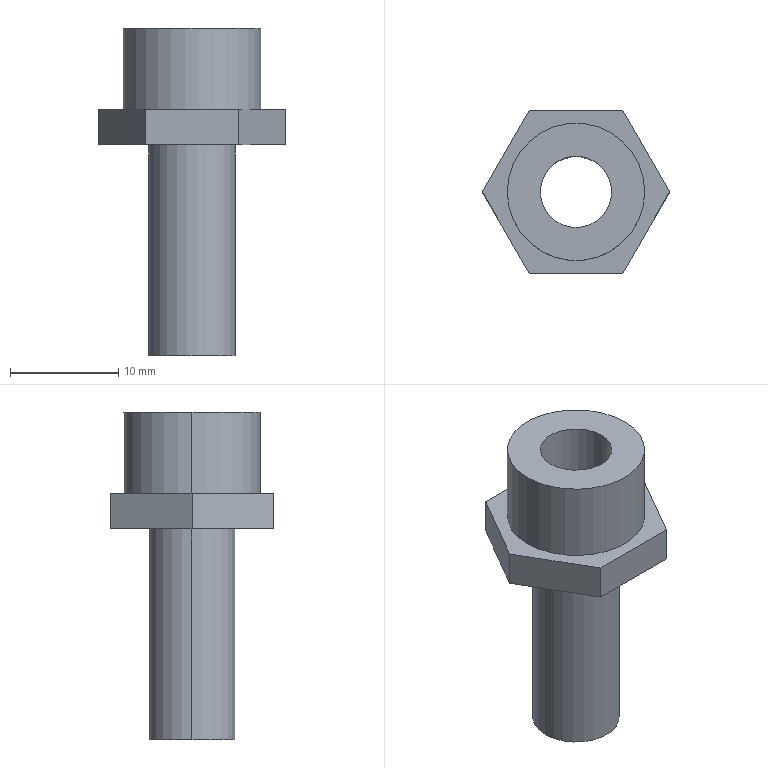Part | STEP file | 2 fen male thread×8mm | 1 solid | 16 faces | box 17.321 x 15 x 30.3 mm | volume 1537 mm3 | plane 10 | cylinder 6 | commonest cylinder face diameters 6.6 x2 8 x2 12.7 x2
STEP:
#1=CARTESIAN_POINT('',(3.3,0.,10.8));
#2=VERTEX_POINT('',#1);
#3=CARTESIAN_POINT('',(-3.3,0.,10.8));
#4=VERTEX_POINT('',#3);
#5=CARTESIAN_POINT('',(0.,0.,10.8));
#6=DIRECTION('',(0.,0.,-1.));
#7=DIRECTION('',(1.,0.,0.));
#8=AXIS2_PLACEMENT_3D('',#5,#6,#7);
#9=CIRCLE('',#8,3.3);
#10=EDGE_CURVE('',#2,#4,#9,.T.);
#11=ORIENTED_EDGE('',*,*,#10,.F.);
#12=CARTESIAN_POINT('',(3.3,0.,-19.5));
#13=VERTEX_POINT('',#12);
#14=CARTESIAN_POINT('',(3.3,0.,10.801));
#15=DIRECTION('',(0.,0.,-1.));
#16=VECTOR('',#15,1000.);
#17=LINE('',#14,#16);
#18=EDGE_CURVE('',#2,#13,#17,.T.);
#19=ORIENTED_EDGE('',*,*,#18,.T.);
#20=CARTESIAN_POINT('',(-3.3,0.,-19.5));
#21=VERTEX_POINT('',#20);
#22=CARTESIAN_POINT('',(0.,0.,-19.5));
#23=DIRECTION('',(0.,0.,-1.));
#24=DIRECTION('',(-1.,0.,0.));
#25=AXIS2_PLACEMENT_3D('',#22,#23,#24);
#26=CIRCLE('',#25,3.3);
#27=EDGE_CURVE('',#13,#21,#26,.T.);
#28=ORIENTED_EDGE('',*,*,#27,.T.);
#29=CARTESIAN_POINT('',(-3.3,0.,10.801));
#30=DIRECTION('',(0.,0.,-1.));
#31=VECTOR('',#30,1000.);
#32=LINE('',#29,#31);
#33=EDGE_CURVE('',#4,#21,#32,.T.);
#34=ORIENTED_EDGE('',*,*,#33,.F.);
#35=EDGE_LOOP('',(#11,#19,#28,#34));
#36=FACE_OUTER_BOUND('',#35,.T.);
#37=CARTESIAN_POINT('',(0.,0.,10.801));
#38=DIRECTION('',(0.,0.,-1.));
#39=DIRECTION('',(-1.,0.,0.));
#40=AXIS2_PLACEMENT_3D('',#37,#38,#39);
#41=CYLINDRICAL_SURFACE('',#40,3.3);
#42=ADVANCED_FACE('',(#36),#41,.F.);
#43=CARTESIAN_POINT('',(-4.,0.,-19.5));
#44=VERTEX_POINT('',#43);
#45=CARTESIAN_POINT('',(4.,0.,-19.5));
#46=VERTEX_POINT('',#45);
#47=CARTESIAN_POINT('',(0.,0.,-19.5));
#48=DIRECTION('',(0.,0.,-1.));
#49=DIRECTION('',(-1.,0.,0.));
#50=AXIS2_PLACEMENT_3D('',#47,#48,#49);
#51=CIRCLE('',#50,4.);
#52=EDGE_CURVE('',#44,#46,#51,.T.);
#53=ORIENTED_EDGE('',*,*,#52,.F.);
#54=CARTESIAN_POINT('',(-4.,0.,0.));
#55=VERTEX_POINT('',#54);
#56=CARTESIAN_POINT('',(-4.,0.,-19.5));
#57=DIRECTION('',(0.,0.,1.));
#58=VECTOR('',#57,1000.);
#59=LINE('',#56,#58);
#60=EDGE_CURVE('',#44,#55,#59,.T.);
#61=ORIENTED_EDGE('',*,*,#60,.T.);
#62=CARTESIAN_POINT('',(4.,0.,0.));
#63=VERTEX_POINT('',#62);
#64=CARTESIAN_POINT('',(0.,0.,0.));
#65=DIRECTION('',(0.,0.,-1.));
#66=DIRECTION('',(-1.,0.,0.));
#67=AXIS2_PLACEMENT_3D('',#64,#65,#66);
#68=CIRCLE('',#67,4.);
#69=EDGE_CURVE('',#55,#63,#68,.T.);
#70=ORIENTED_EDGE('',*,*,#69,.T.);
#71=CARTESIAN_POINT('',(4.,0.,-19.5));
#72=DIRECTION('',(0.,0.,1.));
#73=VECTOR('',#72,1000.);
#74=LINE('',#71,#73);
#75=EDGE_CURVE('',#46,#63,#74,.T.);
#76=ORIENTED_EDGE('',*,*,#75,.F.);
#77=EDGE_LOOP('',(#53,#61,#70,#76));
#78=FACE_OUTER_BOUND('',#77,.T.);
#79=CARTESIAN_POINT('',(0.,0.,-19.5));
#80=DIRECTION('',(0.,0.,1.));
#81=DIRECTION('',(1.,0.,0.));
#82=AXIS2_PLACEMENT_3D('',#79,#80,#81);
#83=CYLINDRICAL_SURFACE('',#82,4.);
#84=ADVANCED_FACE('',(#78),#83,.T.);
#85=CARTESIAN_POINT('',(6.35,0.,10.8));
#86=VERTEX_POINT('',#85);
#87=CARTESIAN_POINT('',(-6.35,0.,10.8));
#88=VERTEX_POINT('',#87);
#89=CARTESIAN_POINT('',(0.,0.,10.8));
#90=DIRECTION('',(0.,0.,1.));
#91=DIRECTION('',(1.,0.,0.));
#92=AXIS2_PLACEMENT_3D('',#89,#90,#91);
#93=CIRCLE('',#92,6.35);
#94=EDGE_CURVE('',#86,#88,#93,.T.);
#95=ORIENTED_EDGE('',*,*,#94,.F.);
#96=CARTESIAN_POINT('',(6.35,0.,3.3));
#97=VERTEX_POINT('',#96);
#98=CARTESIAN_POINT('',(6.35,0.,10.8));
#99=DIRECTION('',(0.,0.,-1.));
#100=VECTOR('',#99,1000.);
#101=LINE('',#98,#100);
#102=EDGE_CURVE('',#86,#97,#101,.T.);
#103=ORIENTED_EDGE('',*,*,#102,.T.);
#104=CARTESIAN_POINT('',(-6.35,0.,3.3));
#105=VERTEX_POINT('',#104);
#106=CARTESIAN_POINT('',(0.,0.,3.3));
#107=DIRECTION('',(0.,0.,1.));
#108=DIRECTION('',(1.,0.,0.));
#109=AXIS2_PLACEMENT_3D('',#106,#107,#108);
#110=CIRCLE('',#109,6.35);
#111=EDGE_CURVE('',#97,#105,#110,.T.);
#112=ORIENTED_EDGE('',*,*,#111,.T.);
#113=CARTESIAN_POINT('',(-6.35,0.,10.8));
#114=DIRECTION('',(0.,0.,-1.));
#115=VECTOR('',#114,1000.);
#116=LINE('',#113,#115);
#117=EDGE_CURVE('',#88,#105,#116,.T.);
#118=ORIENTED_EDGE('',*,*,#117,.F.);
#119=EDGE_LOOP('',(#95,#103,#112,#118));
#120=FACE_OUTER_BOUND('',#119,.T.);
#121=CARTESIAN_POINT('',(0.,0.,10.8));
#122=DIRECTION('',(0.,0.,-1.));
#123=DIRECTION('',(-1.,0.,0.));
#124=AXIS2_PLACEMENT_3D('',#121,#122,#123);
#125=CYLINDRICAL_SURFACE('',#124,6.35);
#126=ADVANCED_FACE('',(#120),#125,.T.);
#127=CARTESIAN_POINT('',(4.33,-7.5,0.));
#128=VERTEX_POINT('',#127);
#129=CARTESIAN_POINT('',(8.66,0.,0.));
#130=VERTEX_POINT('',#129);
#131=CARTESIAN_POINT('',(4.33,-7.5,0.));
#132=DIRECTION('',(0.5,0.866,0.));
#133=VECTOR('',#132,1000.);
#134=LINE('',#131,#133);
#135=EDGE_CURVE('',#128,#130,#134,.T.);
#136=ORIENTED_EDGE('',*,*,#135,.T.);
#137=CARTESIAN_POINT('',(8.66,0.,3.3));
#138=VERTEX_POINT('',#137);
#139=CARTESIAN_POINT('',(8.66,0.,3.3));
#140=DIRECTION('',(0.,0.,-1.));
#141=VECTOR('',#140,1000.);
#142=LINE('',#139,#141);
#143=EDGE_CURVE('',#138,#130,#142,.T.);
#144=ORIENTED_EDGE('',*,*,#143,.F.);
#145=CARTESIAN_POINT('',(4.33,-7.5,3.3));
#146=VERTEX_POINT('',#145);
#147=CARTESIAN_POINT('',(4.33,-7.5,3.3));
#148=DIRECTION('',(0.5,0.866,0.));
#149=VECTOR('',#148,1000.);
#150=LINE('',#147,#149);
#151=EDGE_CURVE('',#146,#138,#150,.T.);
#152=ORIENTED_EDGE('',*,*,#151,.F.);
#153=CARTESIAN_POINT('',(4.33,-7.5,3.3));
#154=DIRECTION('',(0.,0.,-1.));
#155=VECTOR('',#154,1000.);
#156=LINE('',#153,#155);
#157=EDGE_CURVE('',#146,#128,#156,.T.);
#158=ORIENTED_EDGE('',*,*,#157,.T.);
#159=EDGE_LOOP('',(#136,#144,#152,#158));
#160=FACE_OUTER_BOUND('',#159,.T.);
#161=CARTESIAN_POINT('',(4.33,-7.5,3.3));
#162=DIRECTION('',(-0.866,0.5,0.));
#163=DIRECTION('',(-0.5,-0.866,0.));
#164=AXIS2_PLACEMENT_3D('',#161,#162,#163);
#165=PLANE('',#164);
#166=ADVANCED_FACE('',(#160),#165,.F.);
#167=CARTESIAN_POINT('',(4.33,7.5,0.));
#168=VERTEX_POINT('',#167);
#169=CARTESIAN_POINT('',(8.66,0.,0.));
#170=DIRECTION('',(-0.5,0.866,0.));
#171=VECTOR('',#170,1000.);
#172=LINE('',#169,#171);
#173=EDGE_CURVE('',#130,#168,#172,.T.);
#174=ORIENTED_EDGE('',*,*,#173,.T.);
#175=CARTESIAN_POINT('',(4.33,7.5,3.3));
#176=VERTEX_POINT('',#175);
#177=CARTESIAN_POINT('',(4.33,7.5,3.3));
#178=DIRECTION('',(0.,0.,-1.));
#179=VECTOR('',#178,1000.);
#180=LINE('',#177,#179);
#181=EDGE_CURVE('',#176,#168,#180,.T.);
#182=ORIENTED_EDGE('',*,*,#181,.F.);
#183=CARTESIAN_POINT('',(8.66,0.,3.3));
#184=DIRECTION('',(-0.5,0.866,0.));
#185=VECTOR('',#184,1000.);
#186=LINE('',#183,#185);
#187=EDGE_CURVE('',#138,#176,#186,.T.);
#188=ORIENTED_EDGE('',*,*,#187,.F.);
#189=ORIENTED_EDGE('',*,*,#143,.T.);
#190=EDGE_LOOP('',(#174,#182,#188,#189));
#191=FACE_OUTER_BOUND('',#190,.T.);
#192=CARTESIAN_POINT('',(8.66,0.,3.3));
#193=DIRECTION('',(-0.866,-0.5,0.));
#194=DIRECTION('',(0.5,-0.866,0.));
#195=AXIS2_PLACEMENT_3D('',#192,#193,#194);
#196=PLANE('',#195);
#197=ADVANCED_FACE('',(#191),#196,.F.);
#198=CARTESIAN_POINT('',(-4.33,7.5,0.));
#199=VERTEX_POINT('',#198);
#200=CARTESIAN_POINT('',(4.33,7.5,0.));
#201=DIRECTION('',(-1.,0.,0.));
#202=VECTOR('',#201,1000.);
#203=LINE('',#200,#202);
#204=EDGE_CURVE('',#168,#199,#203,.T.);
#205=ORIENTED_EDGE('',*,*,#204,.T.);
#206=CARTESIAN_POINT('',(-4.33,7.5,3.3));
#207=VERTEX_POINT('',#206);
#208=CARTESIAN_POINT('',(-4.33,7.5,3.3));
#209=DIRECTION('',(0.,0.,-1.));
#210=VECTOR('',#209,1000.);
#211=LINE('',#208,#210);
#212=EDGE_CURVE('',#207,#199,#211,.T.);
#213=ORIENTED_EDGE('',*,*,#212,.F.);
#214=CARTESIAN_POINT('',(4.33,7.5,3.3));
#215=DIRECTION('',(-1.,0.,0.));
#216=VECTOR('',#215,1000.);
#217=LINE('',#214,#216);
#218=EDGE_CURVE('',#176,#207,#217,.T.);
#219=ORIENTED_EDGE('',*,*,#218,.F.);
#220=ORIENTED_EDGE('',*,*,#181,.T.);
#221=EDGE_LOOP('',(#205,#213,#219,#220));
#222=FACE_OUTER_BOUND('',#221,.T.);
#223=CARTESIAN_POINT('',(4.33,7.5,3.3));
#224=DIRECTION('',(0.,-1.,0.));
#225=DIRECTION('',(1.,0.,0.));
#226=AXIS2_PLACEMENT_3D('',#223,#224,#225);
#227=PLANE('',#226);
#228=ADVANCED_FACE('',(#222),#227,.F.);
#229=CARTESIAN_POINT('',(-8.66,0.,0.));
#230=VERTEX_POINT('',#229);
#231=CARTESIAN_POINT('',(-4.33,7.5,0.));
#232=DIRECTION('',(-0.5,-0.866,0.));
#233=VECTOR('',#232,1000.);
#234=LINE('',#231,#233);
#235=EDGE_CURVE('',#199,#230,#234,.T.);
#236=ORIENTED_EDGE('',*,*,#235,.T.);
#237=CARTESIAN_POINT('',(-8.66,0.,3.3));
#238=VERTEX_POINT('',#237);
#239=CARTESIAN_POINT('',(-8.66,0.,3.3));
#240=DIRECTION('',(0.,0.,-1.));
#241=VECTOR('',#240,1000.);
#242=LINE('',#239,#241);
#243=EDGE_CURVE('',#238,#230,#242,.T.);
#244=ORIENTED_EDGE('',*,*,#243,.F.);
#245=CARTESIAN_POINT('',(-4.33,7.5,3.3));
#246=DIRECTION('',(-0.5,-0.866,0.));
#247=VECTOR('',#246,1000.);
#248=LINE('',#245,#247);
#249=EDGE_CURVE('',#207,#238,#248,.T.);
#250=ORIENTED_EDGE('',*,*,#249,.F.);
#251=ORIENTED_EDGE('',*,*,#212,.T.);
#252=EDGE_LOOP('',(#236,#244,#250,#251));
#253=FACE_OUTER_BOUND('',#252,.T.);
#254=CARTESIAN_POINT('',(-4.33,7.5,3.3));
#255=DIRECTION('',(0.866,-0.5,0.));
#256=DIRECTION('',(0.5,0.866,0.));
#257=AXIS2_PLACEMENT_3D('',#254,#255,#256);
#258=PLANE('',#257);
#259=ADVANCED_FACE('',(#253),#258,.F.);
#260=CARTESIAN_POINT('',(-4.33,-7.5,0.));
#261=VERTEX_POINT('',#260);
#262=CARTESIAN_POINT('',(-8.66,0.,0.));
#263=DIRECTION('',(0.5,-0.866,0.));
#264=VECTOR('',#263,1000.);
#265=LINE('',#262,#264);
#266=EDGE_CURVE('',#230,#261,#265,.T.);
#267=ORIENTED_EDGE('',*,*,#266,.T.);
#268=CARTESIAN_POINT('',(-4.33,-7.5,3.3));
#269=VERTEX_POINT('',#268);
#270=CARTESIAN_POINT('',(-4.33,-7.5,3.3));
#271=DIRECTION('',(0.,0.,-1.));
#272=VECTOR('',#271,1000.);
#273=LINE('',#270,#272);
#274=EDGE_CURVE('',#269,#261,#273,.T.);
#275=ORIENTED_EDGE('',*,*,#274,.F.);
#276=CARTESIAN_POINT('',(-8.66,0.,3.3));
#277=DIRECTION('',(0.5,-0.866,0.));
#278=VECTOR('',#277,1000.);
#279=LINE('',#276,#278);
#280=EDGE_CURVE('',#238,#269,#279,.T.);
#281=ORIENTED_EDGE('',*,*,#280,.F.);
#282=ORIENTED_EDGE('',*,*,#243,.T.);
#283=EDGE_LOOP('',(#267,#275,#281,#282));
#284=FACE_OUTER_BOUND('',#283,.T.);
#285=CARTESIAN_POINT('',(-8.66,0.,3.3));
#286=DIRECTION('',(0.866,0.5,0.));
#287=DIRECTION('',(-0.5,0.866,0.));
#288=AXIS2_PLACEMENT_3D('',#285,#286,#287);
#289=PLANE('',#288);
#290=ADVANCED_FACE('',(#284),#289,.F.);
#291=CARTESIAN_POINT('',(-4.33,-7.5,0.));
#292=DIRECTION('',(1.,0.,0.));
#293=VECTOR('',#292,1000.);
#294=LINE('',#291,#293);
#295=EDGE_CURVE('',#261,#128,#294,.T.);
#296=ORIENTED_EDGE('',*,*,#295,.T.);
#297=ORIENTED_EDGE('',*,*,#157,.F.);
#298=CARTESIAN_POINT('',(-4.33,-7.5,3.3));
#299=DIRECTION('',(1.,0.,0.));
#300=VECTOR('',#299,1000.);
#301=LINE('',#298,#300);
#302=EDGE_CURVE('',#269,#146,#301,.T.);
#303=ORIENTED_EDGE('',*,*,#302,.F.);
#304=ORIENTED_EDGE('',*,*,#274,.T.);
#305=EDGE_LOOP('',(#296,#297,#303,#304));
#306=FACE_OUTER_BOUND('',#305,.T.);
#307=CARTESIAN_POINT('',(-4.33,-7.5,3.3));
#308=DIRECTION('',(0.,1.,0.));
#309=DIRECTION('',(-1.,0.,0.));
#310=AXIS2_PLACEMENT_3D('',#307,#308,#309);
#311=PLANE('',#310);
#312=ADVANCED_FACE('',(#306),#311,.F.);
#313=CARTESIAN_POINT('',(0.,0.,3.3));
#314=DIRECTION('',(0.,0.,1.));
#315=DIRECTION('',(1.,0.,0.));
#316=AXIS2_PLACEMENT_3D('',#313,#314,#315);
#317=CIRCLE('',#316,6.35);
#318=EDGE_CURVE('',#105,#97,#317,.T.);
#319=ORIENTED_EDGE('',*,*,#318,.F.);
#320=ORIENTED_EDGE('',*,*,#111,.F.);
#321=EDGE_LOOP('',(#319,#320));
#322=FACE_BOUND('',#321,.T.);
#323=ORIENTED_EDGE('',*,*,#151,.T.);
#324=ORIENTED_EDGE('',*,*,#187,.T.);
#325=ORIENTED_EDGE('',*,*,#218,.T.);
#326=ORIENTED_EDGE('',*,*,#249,.T.);
#327=ORIENTED_EDGE('',*,*,#280,.T.);
#328=ORIENTED_EDGE('',*,*,#302,.T.);
#329=EDGE_LOOP('',(#323,#324,#325,#326,#327,#328));
#330=FACE_OUTER_BOUND('',#329,.T.);
#331=CARTESIAN_POINT('',(0.,0.,3.3));
#332=DIRECTION('',(0.,0.,1.));
#333=DIRECTION('',(1.,0.,0.));
#334=AXIS2_PLACEMENT_3D('',#331,#332,#333);
#335=PLANE('',#334);
#336=ADVANCED_FACE('',(#322,#330),#335,.T.);
#337=CARTESIAN_POINT('',(0.,0.,0.));
#338=DIRECTION('',(0.,0.,-1.));
#339=DIRECTION('',(-1.,0.,0.));
#340=AXIS2_PLACEMENT_3D('',#337,#338,#339);
#341=CIRCLE('',#340,4.);
#342=EDGE_CURVE('',#63,#55,#341,.T.);
#343=ORIENTED_EDGE('',*,*,#342,.F.);
#344=ORIENTED_EDGE('',*,*,#69,.F.);
#345=EDGE_LOOP('',(#343,#344));
#346=FACE_BOUND('',#345,.T.);
#347=ORIENTED_EDGE('',*,*,#135,.F.);
#348=ORIENTED_EDGE('',*,*,#295,.F.);
#349=ORIENTED_EDGE('',*,*,#266,.F.);
#350=ORIENTED_EDGE('',*,*,#235,.F.);
#351=ORIENTED_EDGE('',*,*,#204,.F.);
#352=ORIENTED_EDGE('',*,*,#173,.F.);
#353=EDGE_LOOP('',(#347,#348,#349,#350,#351,#352));
#354=FACE_OUTER_BOUND('',#353,.T.);
#355=CARTESIAN_POINT('',(0.,0.,0.));
#356=DIRECTION('',(0.,0.,1.));
#357=DIRECTION('',(1.,0.,0.));
#358=AXIS2_PLACEMENT_3D('',#355,#356,#357);
#359=PLANE('',#358);
#360=ADVANCED_FACE('',(#346,#354),#359,.F.);
#361=ORIENTED_EDGE('',*,*,#102,.F.);
#362=CARTESIAN_POINT('',(0.,0.,10.8));
#363=DIRECTION('',(0.,0.,1.));
#364=DIRECTION('',(1.,0.,0.));
#365=AXIS2_PLACEMENT_3D('',#362,#363,#364);
#366=CIRCLE('',#365,6.35);
#367=EDGE_CURVE('',#88,#86,#366,.T.);
#368=ORIENTED_EDGE('',*,*,#367,.F.);
#369=ORIENTED_EDGE('',*,*,#117,.T.);
#370=ORIENTED_EDGE('',*,*,#318,.T.);
#371=EDGE_LOOP('',(#361,#368,#369,#370));
#372=FACE_OUTER_BOUND('',#371,.T.);
#373=CARTESIAN_POINT('',(0.,0.,10.8));
#374=DIRECTION('',(0.,0.,-1.));
#375=DIRECTION('',(-1.,0.,0.));
#376=AXIS2_PLACEMENT_3D('',#373,#374,#375);
#377=CYLINDRICAL_SURFACE('',#376,6.35);
#378=ADVANCED_FACE('',(#372),#377,.T.);
#379=CARTESIAN_POINT('',(0.,0.,10.8));
#380=DIRECTION('',(0.,0.,-1.));
#381=DIRECTION('',(1.,0.,0.));
#382=AXIS2_PLACEMENT_3D('',#379,#380,#381);
#383=CIRCLE('',#382,3.3);
#384=EDGE_CURVE('',#4,#2,#383,.T.);
#385=ORIENTED_EDGE('',*,*,#384,.T.);
#386=ORIENTED_EDGE('',*,*,#10,.T.);
#387=EDGE_LOOP('',(#385,#386));
#388=FACE_BOUND('',#387,.T.);
#389=ORIENTED_EDGE('',*,*,#367,.T.);
#390=ORIENTED_EDGE('',*,*,#94,.T.);
#391=EDGE_LOOP('',(#389,#390));
#392=FACE_OUTER_BOUND('',#391,.T.);
#393=CARTESIAN_POINT('',(0.,0.,10.8));
#394=DIRECTION('',(0.,0.,1.));
#395=DIRECTION('',(1.,0.,0.));
#396=AXIS2_PLACEMENT_3D('',#393,#394,#395);
#397=PLANE('',#396);
#398=ADVANCED_FACE('',(#388,#392),#397,.T.);
#399=ORIENTED_EDGE('',*,*,#60,.F.);
#400=CARTESIAN_POINT('',(0.,0.,-19.5));
#401=DIRECTION('',(0.,0.,-1.));
#402=DIRECTION('',(-1.,0.,0.));
#403=AXIS2_PLACEMENT_3D('',#400,#401,#402);
#404=CIRCLE('',#403,4.);
#405=EDGE_CURVE('',#46,#44,#404,.T.);
#406=ORIENTED_EDGE('',*,*,#405,.F.);
#407=ORIENTED_EDGE('',*,*,#75,.T.);
#408=ORIENTED_EDGE('',*,*,#342,.T.);
#409=EDGE_LOOP('',(#399,#406,#407,#408));
#410=FACE_OUTER_BOUND('',#409,.T.);
#411=CARTESIAN_POINT('',(0.,0.,-19.5));
#412=DIRECTION('',(0.,0.,1.));
#413=DIRECTION('',(1.,0.,0.));
#414=AXIS2_PLACEMENT_3D('',#411,#412,#413);
#415=CYLINDRICAL_SURFACE('',#414,4.);
#416=ADVANCED_FACE('',(#410),#415,.T.);
#417=CARTESIAN_POINT('',(0.,0.,-19.5));
#418=DIRECTION('',(0.,0.,-1.));
#419=DIRECTION('',(-1.,0.,0.));
#420=AXIS2_PLACEMENT_3D('',#417,#418,#419);
#421=CIRCLE('',#420,3.3);
#422=EDGE_CURVE('',#21,#13,#421,.T.);
#423=ORIENTED_EDGE('',*,*,#422,.F.);
#424=ORIENTED_EDGE('',*,*,#27,.F.);
#425=EDGE_LOOP('',(#423,#424));
#426=FACE_BOUND('',#425,.T.);
#427=ORIENTED_EDGE('',*,*,#405,.T.);
#428=ORIENTED_EDGE('',*,*,#52,.T.);
#429=EDGE_LOOP('',(#427,#428));
#430=FACE_OUTER_BOUND('',#429,.T.);
#431=CARTESIAN_POINT('',(0.,0.,-19.5));
#432=DIRECTION('',(0.,0.,-1.));
#433=DIRECTION('',(-1.,0.,0.));
#434=AXIS2_PLACEMENT_3D('',#431,#432,#433);
#435=PLANE('',#434);
#436=ADVANCED_FACE('',(#426,#430),#435,.T.);
#437=ORIENTED_EDGE('',*,*,#18,.F.);
#438=ORIENTED_EDGE('',*,*,#384,.F.);
#439=ORIENTED_EDGE('',*,*,#33,.T.);
#440=ORIENTED_EDGE('',*,*,#422,.T.);
#441=EDGE_LOOP('',(#437,#438,#439,#440));
#442=FACE_OUTER_BOUND('',#441,.T.);
#443=CARTESIAN_POINT('',(0.,0.,10.801));
#444=DIRECTION('',(0.,0.,-1.));
#445=DIRECTION('',(-1.,0.,0.));
#446=AXIS2_PLACEMENT_3D('',#443,#444,#445);
#447=CYLINDRICAL_SURFACE('',#446,3.3);
#448=ADVANCED_FACE('',(#442),#447,.F.);
#449=CLOSED_SHELL('',(#42,#84,#126,#166,#197,#228,#259,#290,#312,#336,#360,#378,#398,#416,#436,#448));
#450=MANIFOLD_SOLID_BREP('',#449);
#451=CARTESIAN_POINT('',(0.,0.,0.));
#452=DIRECTION('',(0.,0.,1.));
#453=DIRECTION('',(1.,0.,0.));
#454=AXIS2_PLACEMENT_3D('',#451,#452,#453);
#455=(LENGTH_UNIT()NAMED_UNIT(*)SI_UNIT(.MILLI.,.METRE.));
#456=UNCERTAINTY_MEASURE_WITH_UNIT(LENGTH_MEASURE(0.00001),#455,'','');
#457=(NAMED_UNIT(*)PLANE_ANGLE_UNIT()SI_UNIT($,.RADIAN.));
#458=(NAMED_UNIT(*)SI_UNIT($,.STERADIAN.)SOLID_ANGLE_UNIT());
#459=(GEOMETRIC_REPRESENTATION_CONTEXT(3)GLOBAL_UNCERTAINTY_ASSIGNED_CONTEXT((#456))GLOBAL_UNIT_ASSIGNED_CONTEXT((#455,#457,#458))REPRESENTATION_CONTEXT('',''));
#460=ADVANCED_BREP_SHAPE_REPRESENTATION('',(#450,#454),#459);